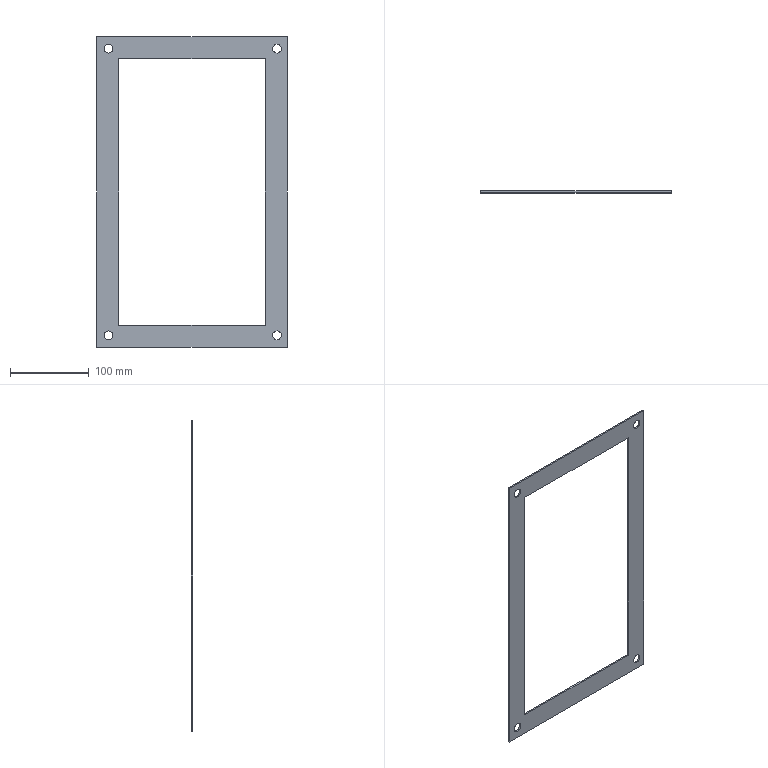Part | SolidWorks | features Extrusion 1, Scale 1 | 1 solid | 18 faces | box 241.875 x 1.875 x 393.75 mm | volume 60360 mm3 | plane 10 | cylinder 8 | commonest cylinder face diameters 11.25 x8
STEP:
#1=CARTESIAN_POINT('',(-82.028,1.438,-292.5));
#2=VERTEX_POINT('',#1);
#3=CARTESIAN_POINT('',(-82.028,1.438,-281.25));
#4=VERTEX_POINT('',#3);
#5=CARTESIAN_POINT('',(-82.028,1.438,-286.875));
#6=DIRECTION('',(0.,1.,0.));
#7=DIRECTION('',(0.,0.,1.));
#8=AXIS2_PLACEMENT_3D('',#5,#6,#7);
#9=CIRCLE('',#8,5.625);
#10=EDGE_CURVE('',#2,#4,#9,.T.);
#11=ORIENTED_EDGE('',*,*,#10,.T.);
#12=CARTESIAN_POINT('',(-82.028,-0.4375,-281.25));
#13=VERTEX_POINT('',#12);
#14=CARTESIAN_POINT('',(-82.028,1.438,-281.25));
#15=DIRECTION('',(0.,-1.,0.));
#16=VECTOR('',#15,1000.);
#17=LINE('',#14,#16);
#18=EDGE_CURVE('',#4,#13,#17,.T.);
#19=ORIENTED_EDGE('',*,*,#18,.T.);
#20=CARTESIAN_POINT('',(-82.028,-0.4375,-292.5));
#21=VERTEX_POINT('',#20);
#22=CARTESIAN_POINT('',(-82.028,-0.4375,-286.875));
#23=DIRECTION('',(0.,1.,0.));
#24=DIRECTION('',(0.,0.,1.));
#25=AXIS2_PLACEMENT_3D('',#22,#23,#24);
#26=CIRCLE('',#25,5.625);
#27=EDGE_CURVE('',#21,#13,#26,.T.);
#28=ORIENTED_EDGE('',*,*,#27,.F.);
#29=CARTESIAN_POINT('',(-82.028,1.438,-292.5));
#30=DIRECTION('',(0.,-1.,0.));
#31=VECTOR('',#30,1000.);
#32=LINE('',#29,#31);
#33=EDGE_CURVE('',#2,#21,#32,.T.);
#34=ORIENTED_EDGE('',*,*,#33,.F.);
#35=EDGE_LOOP('',(#11,#19,#28,#34));
#36=FACE_OUTER_BOUND('',#35,.T.);
#37=CARTESIAN_POINT('',(-82.028,1.438,-286.875));
#38=DIRECTION('',(0.,-1.,0.));
#39=DIRECTION('',(0.,0.,-1.));
#40=AXIS2_PLACEMENT_3D('',#37,#38,#39);
#41=CYLINDRICAL_SURFACE('',#40,5.625);
#42=ADVANCED_FACE('',(#36),#41,.F.);
#43=CARTESIAN_POINT('',(131.722,1.438,-292.5));
#44=VERTEX_POINT('',#43);
#45=CARTESIAN_POINT('',(131.722,1.438,-281.25));
#46=VERTEX_POINT('',#45);
#47=CARTESIAN_POINT('',(131.722,1.438,-286.875));
#48=DIRECTION('',(0.,1.,0.));
#49=DIRECTION('',(0.,0.,1.));
#50=AXIS2_PLACEMENT_3D('',#47,#48,#49);
#51=CIRCLE('',#50,5.625);
#52=EDGE_CURVE('',#44,#46,#51,.T.);
#53=ORIENTED_EDGE('',*,*,#52,.T.);
#54=CARTESIAN_POINT('',(131.722,-0.4375,-281.25));
#55=VERTEX_POINT('',#54);
#56=CARTESIAN_POINT('',(131.722,1.438,-281.25));
#57=DIRECTION('',(0.,-1.,0.));
#58=VECTOR('',#57,1000.);
#59=LINE('',#56,#58);
#60=EDGE_CURVE('',#46,#55,#59,.T.);
#61=ORIENTED_EDGE('',*,*,#60,.T.);
#62=CARTESIAN_POINT('',(131.722,-0.4375,-292.5));
#63=VERTEX_POINT('',#62);
#64=CARTESIAN_POINT('',(131.722,-0.4375,-286.875));
#65=DIRECTION('',(0.,1.,0.));
#66=DIRECTION('',(0.,0.,1.));
#67=AXIS2_PLACEMENT_3D('',#64,#65,#66);
#68=CIRCLE('',#67,5.625);
#69=EDGE_CURVE('',#63,#55,#68,.T.);
#70=ORIENTED_EDGE('',*,*,#69,.F.);
#71=CARTESIAN_POINT('',(131.722,1.438,-292.5));
#72=DIRECTION('',(0.,-1.,0.));
#73=VECTOR('',#72,1000.);
#74=LINE('',#71,#73);
#75=EDGE_CURVE('',#44,#63,#74,.T.);
#76=ORIENTED_EDGE('',*,*,#75,.F.);
#77=EDGE_LOOP('',(#53,#61,#70,#76));
#78=FACE_OUTER_BOUND('',#77,.T.);
#79=CARTESIAN_POINT('',(131.722,1.438,-286.875));
#80=DIRECTION('',(0.,-1.,0.));
#81=DIRECTION('',(0.,0.,-1.));
#82=AXIS2_PLACEMENT_3D('',#79,#80,#81);
#83=CYLINDRICAL_SURFACE('',#82,5.625);
#84=ADVANCED_FACE('',(#78),#83,.F.);
#85=CARTESIAN_POINT('',(131.722,1.438,71.25));
#86=VERTEX_POINT('',#85);
#87=CARTESIAN_POINT('',(131.722,1.438,82.5));
#88=VERTEX_POINT('',#87);
#89=CARTESIAN_POINT('',(131.722,1.438,76.875));
#90=DIRECTION('',(0.,1.,0.));
#91=DIRECTION('',(0.,0.,1.));
#92=AXIS2_PLACEMENT_3D('',#89,#90,#91);
#93=CIRCLE('',#92,5.625);
#94=EDGE_CURVE('',#86,#88,#93,.T.);
#95=ORIENTED_EDGE('',*,*,#94,.T.);
#96=CARTESIAN_POINT('',(131.722,-0.4375,82.5));
#97=VERTEX_POINT('',#96);
#98=CARTESIAN_POINT('',(131.722,1.438,82.5));
#99=DIRECTION('',(0.,-1.,0.));
#100=VECTOR('',#99,1000.);
#101=LINE('',#98,#100);
#102=EDGE_CURVE('',#88,#97,#101,.T.);
#103=ORIENTED_EDGE('',*,*,#102,.T.);
#104=CARTESIAN_POINT('',(131.722,-0.4375,71.25));
#105=VERTEX_POINT('',#104);
#106=CARTESIAN_POINT('',(131.722,-0.4375,76.875));
#107=DIRECTION('',(0.,1.,0.));
#108=DIRECTION('',(0.,0.,1.));
#109=AXIS2_PLACEMENT_3D('',#106,#107,#108);
#110=CIRCLE('',#109,5.625);
#111=EDGE_CURVE('',#105,#97,#110,.T.);
#112=ORIENTED_EDGE('',*,*,#111,.F.);
#113=CARTESIAN_POINT('',(131.722,1.438,71.25));
#114=DIRECTION('',(0.,-1.,0.));
#115=VECTOR('',#114,1000.);
#116=LINE('',#113,#115);
#117=EDGE_CURVE('',#86,#105,#116,.T.);
#118=ORIENTED_EDGE('',*,*,#117,.F.);
#119=EDGE_LOOP('',(#95,#103,#112,#118));
#120=FACE_OUTER_BOUND('',#119,.T.);
#121=CARTESIAN_POINT('',(131.722,1.438,76.875));
#122=DIRECTION('',(0.,-1.,0.));
#123=DIRECTION('',(0.,0.,-1.));
#124=AXIS2_PLACEMENT_3D('',#121,#122,#123);
#125=CYLINDRICAL_SURFACE('',#124,5.625);
#126=ADVANCED_FACE('',(#120),#125,.F.);
#127=CARTESIAN_POINT('',(-82.028,1.438,71.25));
#128=VERTEX_POINT('',#127);
#129=CARTESIAN_POINT('',(-82.028,1.438,82.5));
#130=VERTEX_POINT('',#129);
#131=CARTESIAN_POINT('',(-82.028,1.438,76.875));
#132=DIRECTION('',(0.,1.,0.));
#133=DIRECTION('',(0.,0.,1.));
#134=AXIS2_PLACEMENT_3D('',#131,#132,#133);
#135=CIRCLE('',#134,5.625);
#136=EDGE_CURVE('',#128,#130,#135,.T.);
#137=ORIENTED_EDGE('',*,*,#136,.T.);
#138=CARTESIAN_POINT('',(-82.028,-0.4375,82.5));
#139=VERTEX_POINT('',#138);
#140=CARTESIAN_POINT('',(-82.028,1.438,82.5));
#141=DIRECTION('',(0.,-1.,0.));
#142=VECTOR('',#141,1000.);
#143=LINE('',#140,#142);
#144=EDGE_CURVE('',#130,#139,#143,.T.);
#145=ORIENTED_EDGE('',*,*,#144,.T.);
#146=CARTESIAN_POINT('',(-82.028,-0.4375,71.25));
#147=VERTEX_POINT('',#146);
#148=CARTESIAN_POINT('',(-82.028,-0.4375,76.875));
#149=DIRECTION('',(0.,1.,0.));
#150=DIRECTION('',(0.,0.,1.));
#151=AXIS2_PLACEMENT_3D('',#148,#149,#150);
#152=CIRCLE('',#151,5.625);
#153=EDGE_CURVE('',#147,#139,#152,.T.);
#154=ORIENTED_EDGE('',*,*,#153,.F.);
#155=CARTESIAN_POINT('',(-82.028,1.438,71.25));
#156=DIRECTION('',(0.,-1.,0.));
#157=VECTOR('',#156,1000.);
#158=LINE('',#155,#157);
#159=EDGE_CURVE('',#128,#147,#158,.T.);
#160=ORIENTED_EDGE('',*,*,#159,.F.);
#161=EDGE_LOOP('',(#137,#145,#154,#160));
#162=FACE_OUTER_BOUND('',#161,.T.);
#163=CARTESIAN_POINT('',(-82.028,1.438,76.875));
#164=DIRECTION('',(0.,-1.,0.));
#165=DIRECTION('',(0.,0.,-1.));
#166=AXIS2_PLACEMENT_3D('',#163,#164,#165);
#167=CYLINDRICAL_SURFACE('',#166,5.625);
#168=ADVANCED_FACE('',(#162),#167,.F.);
#169=ORIENTED_EDGE('',*,*,#52,.F.);
#170=CARTESIAN_POINT('',(131.722,1.438,-286.875));
#171=DIRECTION('',(0.,1.,0.));
#172=DIRECTION('',(0.,0.,1.));
#173=AXIS2_PLACEMENT_3D('',#170,#171,#172);
#174=CIRCLE('',#173,5.625);
#175=EDGE_CURVE('',#46,#44,#174,.T.);
#176=ORIENTED_EDGE('',*,*,#175,.F.);
#177=EDGE_LOOP('',(#169,#176));
#178=FACE_BOUND('',#177,.T.);
#179=ORIENTED_EDGE('',*,*,#136,.F.);
#180=CARTESIAN_POINT('',(-82.028,1.438,76.875));
#181=DIRECTION('',(0.,1.,0.));
#182=DIRECTION('',(0.,0.,1.));
#183=AXIS2_PLACEMENT_3D('',#180,#181,#182);
#184=CIRCLE('',#183,5.625);
#185=EDGE_CURVE('',#130,#128,#184,.T.);
#186=ORIENTED_EDGE('',*,*,#185,.F.);
#187=EDGE_LOOP('',(#179,#186));
#188=FACE_BOUND('',#187,.T.);
#189=CARTESIAN_POINT('',(-97.028,1.438,-301.875));
#190=VERTEX_POINT('',#189);
#191=CARTESIAN_POINT('',(-97.028,1.438,91.875));
#192=VERTEX_POINT('',#191);
#193=CARTESIAN_POINT('',(-97.028,1.438,91.875));
#194=DIRECTION('',(0.,0.,1.));
#195=VECTOR('',#194,1000.);
#196=LINE('',#193,#195);
#197=EDGE_CURVE('',#190,#192,#196,.T.);
#198=ORIENTED_EDGE('',*,*,#197,.T.);
#199=CARTESIAN_POINT('',(144.847,1.438,91.875));
#200=VERTEX_POINT('',#199);
#201=CARTESIAN_POINT('',(-97.028,1.438,91.875));
#202=DIRECTION('',(1.,0.,0.));
#203=VECTOR('',#202,1000.);
#204=LINE('',#201,#203);
#205=EDGE_CURVE('',#192,#200,#204,.T.);
#206=ORIENTED_EDGE('',*,*,#205,.T.);
#207=CARTESIAN_POINT('',(144.847,1.438,-301.875));
#208=VERTEX_POINT('',#207);
#209=CARTESIAN_POINT('',(144.847,1.438,91.875));
#210=DIRECTION('',(0.,0.,-1.));
#211=VECTOR('',#210,1000.);
#212=LINE('',#209,#211);
#213=EDGE_CURVE('',#200,#208,#212,.T.);
#214=ORIENTED_EDGE('',*,*,#213,.T.);
#215=CARTESIAN_POINT('',(-97.028,1.438,-301.875));
#216=DIRECTION('',(-1.,0.,0.));
#217=VECTOR('',#216,1000.);
#218=LINE('',#215,#217);
#219=EDGE_CURVE('',#208,#190,#218,.T.);
#220=ORIENTED_EDGE('',*,*,#219,.T.);
#221=EDGE_LOOP('',(#198,#206,#214,#220));
#222=FACE_OUTER_BOUND('',#221,.T.);
#223=CARTESIAN_POINT('',(-68.903,1.438,63.75));
#224=VERTEX_POINT('',#223);
#225=CARTESIAN_POINT('',(116.722,1.438,63.75));
#226=VERTEX_POINT('',#225);
#227=CARTESIAN_POINT('',(-68.903,1.438,63.75));
#228=DIRECTION('',(1.,0.,0.));
#229=VECTOR('',#228,1000.);
#230=LINE('',#227,#229);
#231=EDGE_CURVE('',#224,#226,#230,.T.);
#232=ORIENTED_EDGE('',*,*,#231,.F.);
#233=CARTESIAN_POINT('',(-68.903,1.438,-273.75));
#234=VERTEX_POINT('',#233);
#235=CARTESIAN_POINT('',(-68.903,1.438,63.75));
#236=DIRECTION('',(0.,0.,1.));
#237=VECTOR('',#236,1000.);
#238=LINE('',#235,#237);
#239=EDGE_CURVE('',#234,#224,#238,.T.);
#240=ORIENTED_EDGE('',*,*,#239,.F.);
#241=CARTESIAN_POINT('',(116.722,1.438,-273.75));
#242=VERTEX_POINT('',#241);
#243=CARTESIAN_POINT('',(-68.903,1.438,-273.75));
#244=DIRECTION('',(-1.,0.,0.));
#245=VECTOR('',#244,1000.);
#246=LINE('',#243,#245);
#247=EDGE_CURVE('',#242,#234,#246,.T.);
#248=ORIENTED_EDGE('',*,*,#247,.F.);
#249=CARTESIAN_POINT('',(116.722,1.438,63.75));
#250=DIRECTION('',(0.,0.,-1.));
#251=VECTOR('',#250,1000.);
#252=LINE('',#249,#251);
#253=EDGE_CURVE('',#226,#242,#252,.T.);
#254=ORIENTED_EDGE('',*,*,#253,.F.);
#255=EDGE_LOOP('',(#232,#240,#248,#254));
#256=FACE_BOUND('',#255,.T.);
#257=ORIENTED_EDGE('',*,*,#94,.F.);
#258=CARTESIAN_POINT('',(131.722,1.438,76.875));
#259=DIRECTION('',(0.,1.,0.));
#260=DIRECTION('',(0.,0.,1.));
#261=AXIS2_PLACEMENT_3D('',#258,#259,#260);
#262=CIRCLE('',#261,5.625);
#263=EDGE_CURVE('',#88,#86,#262,.T.);
#264=ORIENTED_EDGE('',*,*,#263,.F.);
#265=EDGE_LOOP('',(#257,#264));
#266=FACE_BOUND('',#265,.T.);
#267=ORIENTED_EDGE('',*,*,#10,.F.);
#268=CARTESIAN_POINT('',(-82.028,1.438,-286.875));
#269=DIRECTION('',(0.,1.,0.));
#270=DIRECTION('',(0.,0.,1.));
#271=AXIS2_PLACEMENT_3D('',#268,#269,#270);
#272=CIRCLE('',#271,5.625);
#273=EDGE_CURVE('',#4,#2,#272,.T.);
#274=ORIENTED_EDGE('',*,*,#273,.F.);
#275=EDGE_LOOP('',(#267,#274));
#276=FACE_BOUND('',#275,.T.);
#277=CARTESIAN_POINT('',(-20.91,1.438,91.875));
#278=DIRECTION('',(0.,-1.,0.));
#279=DIRECTION('',(0.,0.,-1.));
#280=AXIS2_PLACEMENT_3D('',#277,#278,#279);
#281=PLANE('',#280);
#282=ADVANCED_FACE('',(#178,#188,#222,#256,#266,#276),#281,.F.);
#283=ORIENTED_EDGE('',*,*,#69,.T.);
#284=CARTESIAN_POINT('',(131.722,-0.4375,-286.875));
#285=DIRECTION('',(0.,1.,0.));
#286=DIRECTION('',(0.,0.,1.));
#287=AXIS2_PLACEMENT_3D('',#284,#285,#286);
#288=CIRCLE('',#287,5.625);
#289=EDGE_CURVE('',#55,#63,#288,.T.);
#290=ORIENTED_EDGE('',*,*,#289,.T.);
#291=EDGE_LOOP('',(#283,#290));
#292=FACE_BOUND('',#291,.T.);
#293=ORIENTED_EDGE('',*,*,#153,.T.);
#294=CARTESIAN_POINT('',(-82.028,-0.4375,76.875));
#295=DIRECTION('',(0.,1.,0.));
#296=DIRECTION('',(0.,0.,1.));
#297=AXIS2_PLACEMENT_3D('',#294,#295,#296);
#298=CIRCLE('',#297,5.625);
#299=EDGE_CURVE('',#139,#147,#298,.T.);
#300=ORIENTED_EDGE('',*,*,#299,.T.);
#301=EDGE_LOOP('',(#293,#300));
#302=FACE_BOUND('',#301,.T.);
#303=CARTESIAN_POINT('',(-97.028,-0.4375,-301.875));
#304=VERTEX_POINT('',#303);
#305=CARTESIAN_POINT('',(-97.028,-0.4375,91.875));
#306=VERTEX_POINT('',#305);
#307=CARTESIAN_POINT('',(-97.028,-0.4375,91.875));
#308=DIRECTION('',(0.,0.,1.));
#309=VECTOR('',#308,1000.);
#310=LINE('',#307,#309);
#311=EDGE_CURVE('',#304,#306,#310,.T.);
#312=ORIENTED_EDGE('',*,*,#311,.F.);
#313=CARTESIAN_POINT('',(144.847,-0.4375,-301.875));
#314=VERTEX_POINT('',#313);
#315=CARTESIAN_POINT('',(-97.028,-0.4375,-301.875));
#316=DIRECTION('',(-1.,0.,0.));
#317=VECTOR('',#316,1000.);
#318=LINE('',#315,#317);
#319=EDGE_CURVE('',#314,#304,#318,.T.);
#320=ORIENTED_EDGE('',*,*,#319,.F.);
#321=CARTESIAN_POINT('',(144.847,-0.4375,91.875));
#322=VERTEX_POINT('',#321);
#323=CARTESIAN_POINT('',(144.847,-0.4375,91.875));
#324=DIRECTION('',(0.,0.,-1.));
#325=VECTOR('',#324,1000.);
#326=LINE('',#323,#325);
#327=EDGE_CURVE('',#322,#314,#326,.T.);
#328=ORIENTED_EDGE('',*,*,#327,.F.);
#329=CARTESIAN_POINT('',(-97.028,-0.4375,91.875));
#330=DIRECTION('',(1.,0.,0.));
#331=VECTOR('',#330,1000.);
#332=LINE('',#329,#331);
#333=EDGE_CURVE('',#306,#322,#332,.T.);
#334=ORIENTED_EDGE('',*,*,#333,.F.);
#335=EDGE_LOOP('',(#312,#320,#328,#334));
#336=FACE_OUTER_BOUND('',#335,.T.);
#337=CARTESIAN_POINT('',(-68.903,-0.4375,-273.75));
#338=VERTEX_POINT('',#337);
#339=CARTESIAN_POINT('',(-68.903,-0.4375,63.75));
#340=VERTEX_POINT('',#339);
#341=CARTESIAN_POINT('',(-68.903,-0.4375,63.75));
#342=DIRECTION('',(0.,0.,1.));
#343=VECTOR('',#342,1000.);
#344=LINE('',#341,#343);
#345=EDGE_CURVE('',#338,#340,#344,.T.);
#346=ORIENTED_EDGE('',*,*,#345,.T.);
#347=CARTESIAN_POINT('',(116.722,-0.4375,63.75));
#348=VERTEX_POINT('',#347);
#349=CARTESIAN_POINT('',(-68.903,-0.4375,63.75));
#350=DIRECTION('',(1.,0.,0.));
#351=VECTOR('',#350,1000.);
#352=LINE('',#349,#351);
#353=EDGE_CURVE('',#340,#348,#352,.T.);
#354=ORIENTED_EDGE('',*,*,#353,.T.);
#355=CARTESIAN_POINT('',(116.722,-0.4375,-273.75));
#356=VERTEX_POINT('',#355);
#357=CARTESIAN_POINT('',(116.722,-0.4375,63.75));
#358=DIRECTION('',(0.,0.,-1.));
#359=VECTOR('',#358,1000.);
#360=LINE('',#357,#359);
#361=EDGE_CURVE('',#348,#356,#360,.T.);
#362=ORIENTED_EDGE('',*,*,#361,.T.);
#363=CARTESIAN_POINT('',(-68.903,-0.4375,-273.75));
#364=DIRECTION('',(-1.,0.,0.));
#365=VECTOR('',#364,1000.);
#366=LINE('',#363,#365);
#367=EDGE_CURVE('',#356,#338,#366,.T.);
#368=ORIENTED_EDGE('',*,*,#367,.T.);
#369=EDGE_LOOP('',(#346,#354,#362,#368));
#370=FACE_BOUND('',#369,.T.);
#371=ORIENTED_EDGE('',*,*,#111,.T.);
#372=CARTESIAN_POINT('',(131.722,-0.4375,76.875));
#373=DIRECTION('',(0.,1.,0.));
#374=DIRECTION('',(0.,0.,1.));
#375=AXIS2_PLACEMENT_3D('',#372,#373,#374);
#376=CIRCLE('',#375,5.625);
#377=EDGE_CURVE('',#97,#105,#376,.T.);
#378=ORIENTED_EDGE('',*,*,#377,.T.);
#379=EDGE_LOOP('',(#371,#378));
#380=FACE_BOUND('',#379,.T.);
#381=ORIENTED_EDGE('',*,*,#27,.T.);
#382=CARTESIAN_POINT('',(-82.028,-0.4375,-286.875));
#383=DIRECTION('',(0.,1.,0.));
#384=DIRECTION('',(0.,0.,1.));
#385=AXIS2_PLACEMENT_3D('',#382,#383,#384);
#386=CIRCLE('',#385,5.625);
#387=EDGE_CURVE('',#13,#21,#386,.T.);
#388=ORIENTED_EDGE('',*,*,#387,.T.);
#389=EDGE_LOOP('',(#381,#388));
#390=FACE_BOUND('',#389,.T.);
#391=CARTESIAN_POINT('',(-20.91,-0.4375,91.875));
#392=DIRECTION('',(0.,-1.,0.));
#393=DIRECTION('',(0.,0.,-1.));
#394=AXIS2_PLACEMENT_3D('',#391,#392,#393);
#395=PLANE('',#394);
#396=ADVANCED_FACE('',(#292,#302,#336,#370,#380,#390),#395,.T.);
#397=ORIENTED_EDGE('',*,*,#311,.T.);
#398=CARTESIAN_POINT('',(-97.028,1.438,91.875));
#399=DIRECTION('',(0.,-1.,0.));
#400=VECTOR('',#399,1000.);
#401=LINE('',#398,#400);
#402=EDGE_CURVE('',#192,#306,#401,.T.);
#403=ORIENTED_EDGE('',*,*,#402,.F.);
#404=ORIENTED_EDGE('',*,*,#197,.F.);
#405=CARTESIAN_POINT('',(-97.028,1.438,-301.875));
#406=DIRECTION('',(0.,-1.,0.));
#407=VECTOR('',#406,1000.);
#408=LINE('',#405,#407);
#409=EDGE_CURVE('',#190,#304,#408,.T.);
#410=ORIENTED_EDGE('',*,*,#409,.T.);
#411=EDGE_LOOP('',(#397,#403,#404,#410));
#412=FACE_OUTER_BOUND('',#411,.T.);
#413=CARTESIAN_POINT('',(-97.028,1.438,91.875));
#414=DIRECTION('',(1.,0.,0.));
#415=DIRECTION('',(0.,0.,-1.));
#416=AXIS2_PLACEMENT_3D('',#413,#414,#415);
#417=PLANE('',#416);
#418=ADVANCED_FACE('',(#412),#417,.F.);
#419=ORIENTED_EDGE('',*,*,#333,.T.);
#420=CARTESIAN_POINT('',(144.847,1.438,91.875));
#421=DIRECTION('',(0.,-1.,0.));
#422=VECTOR('',#421,1000.);
#423=LINE('',#420,#422);
#424=EDGE_CURVE('',#200,#322,#423,.T.);
#425=ORIENTED_EDGE('',*,*,#424,.F.);
#426=ORIENTED_EDGE('',*,*,#205,.F.);
#427=ORIENTED_EDGE('',*,*,#402,.T.);
#428=EDGE_LOOP('',(#419,#425,#426,#427));
#429=FACE_OUTER_BOUND('',#428,.T.);
#430=CARTESIAN_POINT('',(-97.028,1.438,91.875));
#431=DIRECTION('',(0.,0.,-1.));
#432=DIRECTION('',(-1.,0.,0.));
#433=AXIS2_PLACEMENT_3D('',#430,#431,#432);
#434=PLANE('',#433);
#435=ADVANCED_FACE('',(#429),#434,.F.);
#436=ORIENTED_EDGE('',*,*,#327,.T.);
#437=CARTESIAN_POINT('',(144.847,1.438,-301.875));
#438=DIRECTION('',(0.,-1.,0.));
#439=VECTOR('',#438,1000.);
#440=LINE('',#437,#439);
#441=EDGE_CURVE('',#208,#314,#440,.T.);
#442=ORIENTED_EDGE('',*,*,#441,.F.);
#443=ORIENTED_EDGE('',*,*,#213,.F.);
#444=ORIENTED_EDGE('',*,*,#424,.T.);
#445=EDGE_LOOP('',(#436,#442,#443,#444));
#446=FACE_OUTER_BOUND('',#445,.T.);
#447=CARTESIAN_POINT('',(144.847,1.438,91.875));
#448=DIRECTION('',(-1.,0.,0.));
#449=DIRECTION('',(0.,0.,1.));
#450=AXIS2_PLACEMENT_3D('',#447,#448,#449);
#451=PLANE('',#450);
#452=ADVANCED_FACE('',(#446),#451,.F.);
#453=ORIENTED_EDGE('',*,*,#319,.T.);
#454=ORIENTED_EDGE('',*,*,#409,.F.);
#455=ORIENTED_EDGE('',*,*,#219,.F.);
#456=ORIENTED_EDGE('',*,*,#441,.T.);
#457=EDGE_LOOP('',(#453,#454,#455,#456));
#458=FACE_OUTER_BOUND('',#457,.T.);
#459=CARTESIAN_POINT('',(-97.028,1.438,-301.875));
#460=DIRECTION('',(0.,0.,1.));
#461=DIRECTION('',(1.,0.,0.));
#462=AXIS2_PLACEMENT_3D('',#459,#460,#461);
#463=PLANE('',#462);
#464=ADVANCED_FACE('',(#458),#463,.F.);
#465=ORIENTED_EDGE('',*,*,#353,.F.);
#466=CARTESIAN_POINT('',(-68.903,1.438,63.75));
#467=DIRECTION('',(0.,-1.,0.));
#468=VECTOR('',#467,1000.);
#469=LINE('',#466,#468);
#470=EDGE_CURVE('',#224,#340,#469,.T.);
#471=ORIENTED_EDGE('',*,*,#470,.F.);
#472=ORIENTED_EDGE('',*,*,#231,.T.);
#473=CARTESIAN_POINT('',(116.722,1.438,63.75));
#474=DIRECTION('',(0.,-1.,0.));
#475=VECTOR('',#474,1000.);
#476=LINE('',#473,#475);
#477=EDGE_CURVE('',#226,#348,#476,.T.);
#478=ORIENTED_EDGE('',*,*,#477,.T.);
#479=EDGE_LOOP('',(#465,#471,#472,#478));
#480=FACE_OUTER_BOUND('',#479,.T.);
#481=CARTESIAN_POINT('',(-68.903,1.438,63.75));
#482=DIRECTION('',(0.,0.,-1.));
#483=DIRECTION('',(-1.,0.,0.));
#484=AXIS2_PLACEMENT_3D('',#481,#482,#483);
#485=PLANE('',#484);
#486=ADVANCED_FACE('',(#480),#485,.T.);
#487=ORIENTED_EDGE('',*,*,#361,.F.);
#488=ORIENTED_EDGE('',*,*,#477,.F.);
#489=ORIENTED_EDGE('',*,*,#253,.T.);
#490=CARTESIAN_POINT('',(116.722,1.438,-273.75));
#491=DIRECTION('',(0.,-1.,0.));
#492=VECTOR('',#491,1000.);
#493=LINE('',#490,#492);
#494=EDGE_CURVE('',#242,#356,#493,.T.);
#495=ORIENTED_EDGE('',*,*,#494,.T.);
#496=EDGE_LOOP('',(#487,#488,#489,#495));
#497=FACE_OUTER_BOUND('',#496,.T.);
#498=CARTESIAN_POINT('',(116.722,1.438,63.75));
#499=DIRECTION('',(-1.,0.,0.));
#500=DIRECTION('',(0.,0.,1.));
#501=AXIS2_PLACEMENT_3D('',#498,#499,#500);
#502=PLANE('',#501);
#503=ADVANCED_FACE('',(#497),#502,.T.);
#504=ORIENTED_EDGE('',*,*,#367,.F.);
#505=ORIENTED_EDGE('',*,*,#494,.F.);
#506=ORIENTED_EDGE('',*,*,#247,.T.);
#507=CARTESIAN_POINT('',(-68.903,1.438,-273.75));
#508=DIRECTION('',(0.,-1.,0.));
#509=VECTOR('',#508,1000.);
#510=LINE('',#507,#509);
#511=EDGE_CURVE('',#234,#338,#510,.T.);
#512=ORIENTED_EDGE('',*,*,#511,.T.);
#513=EDGE_LOOP('',(#504,#505,#506,#512));
#514=FACE_OUTER_BOUND('',#513,.T.);
#515=CARTESIAN_POINT('',(-68.903,1.438,-273.75));
#516=DIRECTION('',(0.,0.,1.));
#517=DIRECTION('',(1.,0.,0.));
#518=AXIS2_PLACEMENT_3D('',#515,#516,#517);
#519=PLANE('',#518);
#520=ADVANCED_FACE('',(#514),#519,.T.);
#521=ORIENTED_EDGE('',*,*,#345,.F.);
#522=ORIENTED_EDGE('',*,*,#511,.F.);
#523=ORIENTED_EDGE('',*,*,#239,.T.);
#524=ORIENTED_EDGE('',*,*,#470,.T.);
#525=EDGE_LOOP('',(#521,#522,#523,#524));
#526=FACE_OUTER_BOUND('',#525,.T.);
#527=CARTESIAN_POINT('',(-68.903,1.438,63.75));
#528=DIRECTION('',(1.,0.,0.));
#529=DIRECTION('',(0.,0.,-1.));
#530=AXIS2_PLACEMENT_3D('',#527,#528,#529);
#531=PLANE('',#530);
#532=ADVANCED_FACE('',(#526),#531,.T.);
#533=ORIENTED_EDGE('',*,*,#144,.F.);
#534=ORIENTED_EDGE('',*,*,#185,.T.);
#535=ORIENTED_EDGE('',*,*,#159,.T.);
#536=ORIENTED_EDGE('',*,*,#299,.F.);
#537=EDGE_LOOP('',(#533,#534,#535,#536));
#538=FACE_OUTER_BOUND('',#537,.T.);
#539=CARTESIAN_POINT('',(-82.028,1.438,76.875));
#540=DIRECTION('',(0.,-1.,0.));
#541=DIRECTION('',(0.,0.,-1.));
#542=AXIS2_PLACEMENT_3D('',#539,#540,#541);
#543=CYLINDRICAL_SURFACE('',#542,5.625);
#544=ADVANCED_FACE('',(#538),#543,.F.);
#545=ORIENTED_EDGE('',*,*,#102,.F.);
#546=ORIENTED_EDGE('',*,*,#263,.T.);
#547=ORIENTED_EDGE('',*,*,#117,.T.);
#548=ORIENTED_EDGE('',*,*,#377,.F.);
#549=EDGE_LOOP('',(#545,#546,#547,#548));
#550=FACE_OUTER_BOUND('',#549,.T.);
#551=CARTESIAN_POINT('',(131.722,1.438,76.875));
#552=DIRECTION('',(0.,-1.,0.));
#553=DIRECTION('',(0.,0.,-1.));
#554=AXIS2_PLACEMENT_3D('',#551,#552,#553);
#555=CYLINDRICAL_SURFACE('',#554,5.625);
#556=ADVANCED_FACE('',(#550),#555,.F.);
#557=ORIENTED_EDGE('',*,*,#60,.F.);
#558=ORIENTED_EDGE('',*,*,#175,.T.);
#559=ORIENTED_EDGE('',*,*,#75,.T.);
#560=ORIENTED_EDGE('',*,*,#289,.F.);
#561=EDGE_LOOP('',(#557,#558,#559,#560));
#562=FACE_OUTER_BOUND('',#561,.T.);
#563=CARTESIAN_POINT('',(131.722,1.438,-286.875));
#564=DIRECTION('',(0.,-1.,0.));
#565=DIRECTION('',(0.,0.,-1.));
#566=AXIS2_PLACEMENT_3D('',#563,#564,#565);
#567=CYLINDRICAL_SURFACE('',#566,5.625);
#568=ADVANCED_FACE('',(#562),#567,.F.);
#569=ORIENTED_EDGE('',*,*,#18,.F.);
#570=ORIENTED_EDGE('',*,*,#273,.T.);
#571=ORIENTED_EDGE('',*,*,#33,.T.);
#572=ORIENTED_EDGE('',*,*,#387,.F.);
#573=EDGE_LOOP('',(#569,#570,#571,#572));
#574=FACE_OUTER_BOUND('',#573,.T.);
#575=CARTESIAN_POINT('',(-82.028,1.438,-286.875));
#576=DIRECTION('',(0.,-1.,0.));
#577=DIRECTION('',(0.,0.,-1.));
#578=AXIS2_PLACEMENT_3D('',#575,#576,#577);
#579=CYLINDRICAL_SURFACE('',#578,5.625);
#580=ADVANCED_FACE('',(#574),#579,.F.);
#581=CLOSED_SHELL('',(#42,#84,#126,#168,#282,#396,#418,#435,#452,#464,#486,#503,#520,#532,#544,#556,#568,#580));
#582=MANIFOLD_SOLID_BREP('',#581);
#583=CARTESIAN_POINT('',(0.,0.,0.));
#584=DIRECTION('',(0.,0.,1.));
#585=DIRECTION('',(1.,0.,0.));
#586=AXIS2_PLACEMENT_3D('',#583,#584,#585);
#587=(LENGTH_UNIT()NAMED_UNIT(*)SI_UNIT(.MILLI.,.METRE.));
#588=UNCERTAINTY_MEASURE_WITH_UNIT(LENGTH_MEASURE(0.00001),#587,'','');
#589=(NAMED_UNIT(*)PLANE_ANGLE_UNIT()SI_UNIT($,.RADIAN.));
#590=(NAMED_UNIT(*)SI_UNIT($,.STERADIAN.)SOLID_ANGLE_UNIT());
#591=(GEOMETRIC_REPRESENTATION_CONTEXT(3)GLOBAL_UNCERTAINTY_ASSIGNED_CONTEXT((#588))GLOBAL_UNIT_ASSIGNED_CONTEXT((#587,#589,#590))REPRESENTATION_CONTEXT('',''));
#592=ADVANCED_BREP_SHAPE_REPRESENTATION('',(#582,#586),#591);